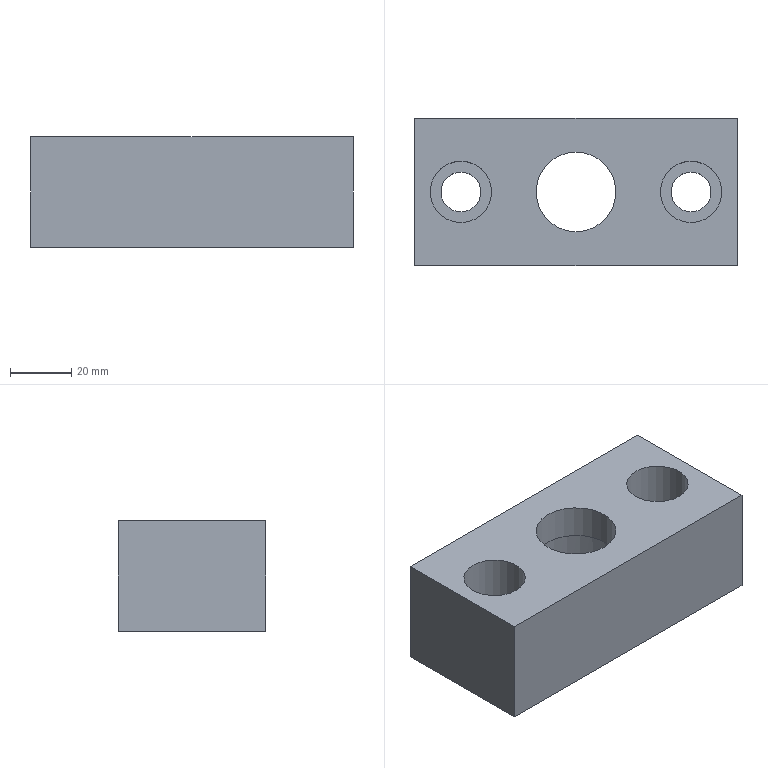Part | NX | features solid 2 | 1 solid | 15 faces | box 105 x 48 x 36 mm | volume 129547 mm3 | plane 9 | cylinder 6 | commonest cylinder face diameters 13 x2 20 x2 26 x1 40 x1
STEP:
#1=CARTESIAN_POINT('',(73.5,-257.,75.));
#2=VERTEX_POINT('',#1);
#3=CARTESIAN_POINT('',(73.5,-237.,75.));
#4=DIRECTION('',(0.,0.,1.));
#5=DIRECTION('',(0.,-1.,0.));
#6=AXIS2_PLACEMENT_3D('',#3,#4,#5);
#7=CIRCLE('',#6,20.);
#8=EDGE_CURVE('',#2,#2,#7,.F.);
#9=ORIENTED_EDGE('',*,*,#8,.T.);
#10=EDGE_LOOP('',(#9));
#11=FACE_BOUND('',#10,.T.);
#12=CARTESIAN_POINT('',(73.5,-250.,75.));
#13=VERTEX_POINT('',#12);
#14=CARTESIAN_POINT('',(73.5,-237.,75.));
#15=DIRECTION('',(0.,0.,1.));
#16=DIRECTION('',(0.,-1.,0.));
#17=AXIS2_PLACEMENT_3D('',#14,#15,#16);
#18=CIRCLE('',#17,13.);
#19=EDGE_CURVE('',#13,#13,#18,.F.);
#20=ORIENTED_EDGE('',*,*,#19,.F.);
#21=EDGE_LOOP('',(#20));
#22=FACE_BOUND('',#21,.T.);
#23=CARTESIAN_POINT('',(73.5,-219.,75.));
#24=DIRECTION('',(0.,0.,-1.));
#25=DIRECTION('',(0.,1.,0.));
#26=AXIS2_PLACEMENT_3D('',#23,#24,#25);
#27=PLANE('',#26);
#28=ADVANCED_FACE('',(#11,#22),#27,.T.);
#29=CARTESIAN_POINT('',(36.,-243.5,72.));
#30=VERTEX_POINT('',#29);
#31=CARTESIAN_POINT('',(36.,-237.,72.));
#32=DIRECTION('',(0.,0.,1.));
#33=DIRECTION('',(0.,-1.,0.));
#34=AXIS2_PLACEMENT_3D('',#31,#32,#33);
#35=CIRCLE('',#34,6.5);
#36=EDGE_CURVE('',#30,#30,#35,.F.);
#37=ORIENTED_EDGE('',*,*,#36,.T.);
#38=EDGE_LOOP('',(#37));
#39=FACE_BOUND('',#38,.T.);
#40=CARTESIAN_POINT('',(36.,-247.,72.));
#41=VERTEX_POINT('',#40);
#42=CARTESIAN_POINT('',(36.,-237.,72.));
#43=DIRECTION('',(0.,0.,1.));
#44=DIRECTION('',(0.,-1.,0.));
#45=AXIS2_PLACEMENT_3D('',#42,#43,#44);
#46=CIRCLE('',#45,10.);
#47=EDGE_CURVE('',#41,#41,#46,.F.);
#48=ORIENTED_EDGE('',*,*,#47,.F.);
#49=EDGE_LOOP('',(#48));
#50=FACE_BOUND('',#49,.T.);
#51=CARTESIAN_POINT('',(36.54,-237.447,72.));
#52=DIRECTION('',(0.,0.,-1.));
#53=DIRECTION('',(0.,-1.,0.));
#54=AXIS2_PLACEMENT_3D('',#51,#52,#53);
#55=PLANE('',#54);
#56=ADVANCED_FACE('',(#39,#50),#55,.F.);
#57=CARTESIAN_POINT('',(73.5,-224.,86.));
#58=VERTEX_POINT('',#57);
#59=CARTESIAN_POINT('',(73.5,-237.,86.));
#60=DIRECTION('',(0.,0.,-1.));
#61=DIRECTION('',(0.,1.,0.));
#62=AXIS2_PLACEMENT_3D('',#59,#60,#61);
#63=CIRCLE('',#62,13.);
#64=EDGE_CURVE('',#58,#58,#63,.F.);
#65=ORIENTED_EDGE('',*,*,#64,.T.);
#66=EDGE_LOOP('',(#65));
#67=FACE_BOUND('',#66,.T.);
#68=ORIENTED_EDGE('',*,*,#19,.T.);
#69=EDGE_LOOP('',(#68));
#70=FACE_BOUND('',#69,.T.);
#71=CARTESIAN_POINT('',(73.5,-237.,29.5));
#72=DIRECTION('',(0.,0.,1.));
#73=DIRECTION('',(0.,1.,0.));
#74=AXIS2_PLACEMENT_3D('',#71,#72,#73);
#75=CYLINDRICAL_SURFACE('',#74,13.);
#76=ADVANCED_FACE('',(#67,#70),#75,.F.);
#77=CARTESIAN_POINT('',(73.5,-217.,50.));
#78=VERTEX_POINT('',#77);
#79=CARTESIAN_POINT('',(73.5,-237.,50.));
#80=DIRECTION('',(0.,0.,-1.));
#81=DIRECTION('',(0.,1.,0.));
#82=AXIS2_PLACEMENT_3D('',#79,#80,#81);
#83=CIRCLE('',#82,20.);
#84=EDGE_CURVE('',#78,#78,#83,.T.);
#85=ORIENTED_EDGE('',*,*,#84,.T.);
#86=EDGE_LOOP('',(#85));
#87=FACE_BOUND('',#86,.T.);
#88=ORIENTED_EDGE('',*,*,#8,.F.);
#89=EDGE_LOOP('',(#88));
#90=FACE_BOUND('',#89,.T.);
#91=CARTESIAN_POINT('',(73.5,-237.,29.));
#92=DIRECTION('',(0.,0.,1.));
#93=DIRECTION('',(0.,1.,0.));
#94=AXIS2_PLACEMENT_3D('',#91,#92,#93);
#95=CYLINDRICAL_SURFACE('',#94,20.);
#96=ADVANCED_FACE('',(#87,#90),#95,.F.);
#97=CARTESIAN_POINT('',(126.,-261.,50.));
#98=VERTEX_POINT('',#97);
#99=CARTESIAN_POINT('',(126.,-261.,86.));
#100=VERTEX_POINT('',#99);
#101=CARTESIAN_POINT('',(126.,-261.,67.5));
#102=DIRECTION('',(0.,0.,1.));
#103=VECTOR('',#102,1000.);
#104=LINE('',#101,#103);
#105=EDGE_CURVE('',#98,#100,#104,.T.);
#106=ORIENTED_EDGE('',*,*,#105,.F.);
#107=CARTESIAN_POINT('',(126.,-213.,50.));
#108=VERTEX_POINT('',#107);
#109=CARTESIAN_POINT('',(126.,-237.,50.));
#110=DIRECTION('',(0.,1.,0.));
#111=VECTOR('',#110,1000.);
#112=LINE('',#109,#111);
#113=EDGE_CURVE('',#108,#98,#112,.F.);
#114=ORIENTED_EDGE('',*,*,#113,.F.);
#115=CARTESIAN_POINT('',(126.,-213.,86.));
#116=VERTEX_POINT('',#115);
#117=CARTESIAN_POINT('',(126.,-213.,67.5));
#118=DIRECTION('',(0.,0.,1.));
#119=VECTOR('',#118,1000.);
#120=LINE('',#117,#119);
#121=EDGE_CURVE('',#108,#116,#120,.T.);
#122=ORIENTED_EDGE('',*,*,#121,.T.);
#123=CARTESIAN_POINT('',(126.,-237.,86.));
#124=DIRECTION('',(0.,1.,0.));
#125=VECTOR('',#124,1000.);
#126=LINE('',#123,#125);
#127=EDGE_CURVE('',#100,#116,#126,.T.);
#128=ORIENTED_EDGE('',*,*,#127,.F.);
#129=EDGE_LOOP('',(#106,#114,#122,#128));
#130=FACE_BOUND('',#129,.T.);
#131=CARTESIAN_POINT('',(126.,-237.,67.5));
#132=DIRECTION('',(1.,0.,0.));
#133=DIRECTION('',(0.,0.,1.));
#134=AXIS2_PLACEMENT_3D('',#131,#132,#133);
#135=PLANE('',#134);
#136=ADVANCED_FACE('',(#130),#135,.T.);
#137=CARTESIAN_POINT('',(21.,-261.,50.));
#138=VERTEX_POINT('',#137);
#139=CARTESIAN_POINT('',(21.,-261.,86.));
#140=VERTEX_POINT('',#139);
#141=CARTESIAN_POINT('',(21.,-261.,67.5));
#142=DIRECTION('',(0.,0.,1.));
#143=VECTOR('',#142,1000.);
#144=LINE('',#141,#143);
#145=EDGE_CURVE('',#138,#140,#144,.T.);
#146=ORIENTED_EDGE('',*,*,#145,.F.);
#147=CARTESIAN_POINT('',(73.5,-261.,50.));
#148=DIRECTION('',(1.,0.,0.));
#149=VECTOR('',#148,1000.);
#150=LINE('',#147,#149);
#151=EDGE_CURVE('',#98,#138,#150,.F.);
#152=ORIENTED_EDGE('',*,*,#151,.F.);
#153=ORIENTED_EDGE('',*,*,#105,.T.);
#154=CARTESIAN_POINT('',(73.5,-261.,86.));
#155=DIRECTION('',(1.,0.,0.));
#156=VECTOR('',#155,1000.);
#157=LINE('',#154,#156);
#158=EDGE_CURVE('',#140,#100,#157,.T.);
#159=ORIENTED_EDGE('',*,*,#158,.F.);
#160=EDGE_LOOP('',(#146,#152,#153,#159));
#161=FACE_BOUND('',#160,.T.);
#162=CARTESIAN_POINT('',(73.5,-261.,67.5));
#163=DIRECTION('',(0.,-1.,0.));
#164=DIRECTION('',(0.,0.,1.));
#165=AXIS2_PLACEMENT_3D('',#162,#163,#164);
#166=PLANE('',#165);
#167=ADVANCED_FACE('',(#161),#166,.T.);
#168=CARTESIAN_POINT('',(21.,-213.,50.));
#169=VERTEX_POINT('',#168);
#170=CARTESIAN_POINT('',(21.,-213.,86.));
#171=VERTEX_POINT('',#170);
#172=CARTESIAN_POINT('',(21.,-213.,67.5));
#173=DIRECTION('',(0.,0.,1.));
#174=VECTOR('',#173,1000.);
#175=LINE('',#172,#174);
#176=EDGE_CURVE('',#169,#171,#175,.T.);
#177=ORIENTED_EDGE('',*,*,#176,.F.);
#178=CARTESIAN_POINT('',(21.,-237.,50.));
#179=DIRECTION('',(0.,-1.,0.));
#180=VECTOR('',#179,1000.);
#181=LINE('',#178,#180);
#182=EDGE_CURVE('',#138,#169,#181,.F.);
#183=ORIENTED_EDGE('',*,*,#182,.F.);
#184=ORIENTED_EDGE('',*,*,#145,.T.);
#185=CARTESIAN_POINT('',(21.,-237.,86.));
#186=DIRECTION('',(0.,-1.,0.));
#187=VECTOR('',#186,1000.);
#188=LINE('',#185,#187);
#189=EDGE_CURVE('',#171,#140,#188,.T.);
#190=ORIENTED_EDGE('',*,*,#189,.F.);
#191=EDGE_LOOP('',(#177,#183,#184,#190));
#192=FACE_BOUND('',#191,.T.);
#193=CARTESIAN_POINT('',(21.,-237.,67.5));
#194=DIRECTION('',(-1.,0.,0.));
#195=DIRECTION('',(0.,0.,-1.));
#196=AXIS2_PLACEMENT_3D('',#193,#194,#195);
#197=PLANE('',#196);
#198=ADVANCED_FACE('',(#192),#197,.T.);
#199=CARTESIAN_POINT('',(73.5,-213.,50.));
#200=DIRECTION('',(-1.,0.,0.));
#201=VECTOR('',#200,1000.);
#202=LINE('',#199,#201);
#203=EDGE_CURVE('',#169,#108,#202,.F.);
#204=ORIENTED_EDGE('',*,*,#203,.F.);
#205=ORIENTED_EDGE('',*,*,#176,.T.);
#206=CARTESIAN_POINT('',(73.5,-213.,86.));
#207=DIRECTION('',(-1.,0.,0.));
#208=VECTOR('',#207,1000.);
#209=LINE('',#206,#208);
#210=EDGE_CURVE('',#116,#171,#209,.T.);
#211=ORIENTED_EDGE('',*,*,#210,.F.);
#212=ORIENTED_EDGE('',*,*,#121,.F.);
#213=EDGE_LOOP('',(#204,#205,#211,#212));
#214=FACE_BOUND('',#213,.T.);
#215=CARTESIAN_POINT('',(73.5,-213.,67.5));
#216=DIRECTION('',(0.,1.,0.));
#217=DIRECTION('',(0.,0.,-1.));
#218=AXIS2_PLACEMENT_3D('',#215,#216,#217);
#219=PLANE('',#218);
#220=ADVANCED_FACE('',(#214),#219,.T.);
#221=CARTESIAN_POINT('',(36.,-230.5,50.));
#222=VERTEX_POINT('',#221);
#223=CARTESIAN_POINT('',(36.,-237.,50.));
#224=DIRECTION('',(0.,0.,-1.));
#225=DIRECTION('',(0.,1.,0.));
#226=AXIS2_PLACEMENT_3D('',#223,#224,#225);
#227=CIRCLE('',#226,6.5);
#228=EDGE_CURVE('',#222,#222,#227,.F.);
#229=ORIENTED_EDGE('',*,*,#228,.F.);
#230=EDGE_LOOP('',(#229));
#231=FACE_BOUND('',#230,.T.);
#232=ORIENTED_EDGE('',*,*,#36,.F.);
#233=EDGE_LOOP('',(#232));
#234=FACE_BOUND('',#233,.T.);
#235=CARTESIAN_POINT('',(36.,-237.,36.));
#236=DIRECTION('',(0.,0.,-1.));
#237=DIRECTION('',(0.,-1.,0.));
#238=AXIS2_PLACEMENT_3D('',#235,#236,#237);
#239=CYLINDRICAL_SURFACE('',#238,6.5);
#240=ADVANCED_FACE('',(#231,#234),#239,.F.);
#241=CARTESIAN_POINT('',(111.,-230.5,50.));
#242=VERTEX_POINT('',#241);
#243=CARTESIAN_POINT('',(111.,-237.,50.));
#244=DIRECTION('',(0.,0.,-1.));
#245=DIRECTION('',(0.,1.,0.));
#246=AXIS2_PLACEMENT_3D('',#243,#244,#245);
#247=CIRCLE('',#246,6.5);
#248=EDGE_CURVE('',#242,#242,#247,.F.);
#249=ORIENTED_EDGE('',*,*,#248,.T.);
#250=EDGE_LOOP('',(#249));
#251=FACE_BOUND('',#250,.T.);
#252=ORIENTED_EDGE('',*,*,#228,.T.);
#253=EDGE_LOOP('',(#252));
#254=FACE_BOUND('',#253,.T.);
#255=ORIENTED_EDGE('',*,*,#203,.T.);
#256=ORIENTED_EDGE('',*,*,#113,.T.);
#257=ORIENTED_EDGE('',*,*,#151,.T.);
#258=ORIENTED_EDGE('',*,*,#182,.T.);
#259=EDGE_LOOP('',(#255,#256,#257,#258));
#260=FACE_BOUND('',#259,.T.);
#261=ORIENTED_EDGE('',*,*,#84,.F.);
#262=EDGE_LOOP('',(#261));
#263=FACE_BOUND('',#262,.T.);
#264=CARTESIAN_POINT('',(-296.5,11.379,50.));
#265=DIRECTION('',(0.,0.,1.));
#266=DIRECTION('',(0.,1.,0.));
#267=AXIS2_PLACEMENT_3D('',#264,#265,#266);
#268=PLANE('',#267);
#269=ADVANCED_FACE('',(#251,#254,#260,#263),#268,.F.);
#270=ORIENTED_EDGE('',*,*,#47,.T.);
#271=EDGE_LOOP('',(#270));
#272=FACE_BOUND('',#271,.T.);
#273=CARTESIAN_POINT('',(36.,-247.,86.));
#274=VERTEX_POINT('',#273);
#275=CARTESIAN_POINT('',(36.,-237.,86.));
#276=DIRECTION('',(0.,0.,1.));
#277=DIRECTION('',(0.,-1.,0.));
#278=AXIS2_PLACEMENT_3D('',#275,#276,#277);
#279=CIRCLE('',#278,10.);
#280=EDGE_CURVE('',#274,#274,#279,.T.);
#281=ORIENTED_EDGE('',*,*,#280,.T.);
#282=EDGE_LOOP('',(#281));
#283=FACE_BOUND('',#282,.T.);
#284=CARTESIAN_POINT('',(36.,-237.,86.));
#285=DIRECTION('',(0.,0.,-1.));
#286=DIRECTION('',(0.,-1.,0.));
#287=AXIS2_PLACEMENT_3D('',#284,#285,#286);
#288=CYLINDRICAL_SURFACE('',#287,10.);
#289=ADVANCED_FACE('',(#272,#283),#288,.F.);
#290=CARTESIAN_POINT('',(111.,-227.,86.));
#291=VERTEX_POINT('',#290);
#292=CARTESIAN_POINT('',(111.,-237.,86.));
#293=DIRECTION('',(0.,0.,-1.));
#294=DIRECTION('',(0.,1.,0.));
#295=AXIS2_PLACEMENT_3D('',#292,#293,#294);
#296=CIRCLE('',#295,10.);
#297=EDGE_CURVE('',#291,#291,#296,.T.);
#298=ORIENTED_EDGE('',*,*,#297,.T.);
#299=EDGE_LOOP('',(#298));
#300=FACE_BOUND('',#299,.T.);
#301=ORIENTED_EDGE('',*,*,#280,.F.);
#302=EDGE_LOOP('',(#301));
#303=FACE_BOUND('',#302,.T.);
#304=ORIENTED_EDGE('',*,*,#189,.T.);
#305=ORIENTED_EDGE('',*,*,#158,.T.);
#306=ORIENTED_EDGE('',*,*,#127,.T.);
#307=ORIENTED_EDGE('',*,*,#210,.T.);
#308=EDGE_LOOP('',(#304,#305,#306,#307));
#309=FACE_BOUND('',#308,.T.);
#310=ORIENTED_EDGE('',*,*,#64,.F.);
#311=EDGE_LOOP('',(#310));
#312=FACE_BOUND('',#311,.T.);
#313=CARTESIAN_POINT('',(-211.5,11.379,86.));
#314=DIRECTION('',(0.,0.,1.));
#315=DIRECTION('',(0.,-1.,0.));
#316=AXIS2_PLACEMENT_3D('',#313,#314,#315);
#317=PLANE('',#316);
#318=ADVANCED_FACE('',(#300,#303,#309,#312),#317,.T.);
#319=CARTESIAN_POINT('',(111.,-243.5,72.));
#320=VERTEX_POINT('',#319);
#321=CARTESIAN_POINT('',(111.,-237.,72.));
#322=DIRECTION('',(0.,0.,-1.));
#323=DIRECTION('',(0.,-1.,0.));
#324=AXIS2_PLACEMENT_3D('',#321,#322,#323);
#325=CIRCLE('',#324,6.5);
#326=EDGE_CURVE('',#320,#320,#325,.T.);
#327=ORIENTED_EDGE('',*,*,#326,.T.);
#328=EDGE_LOOP('',(#327));
#329=FACE_BOUND('',#328,.T.);
#330=CARTESIAN_POINT('',(111.,-247.,72.));
#331=VERTEX_POINT('',#330);
#332=CARTESIAN_POINT('',(111.,-237.,72.));
#333=DIRECTION('',(0.,0.,-1.));
#334=DIRECTION('',(0.,-1.,0.));
#335=AXIS2_PLACEMENT_3D('',#332,#333,#334);
#336=CIRCLE('',#335,10.);
#337=EDGE_CURVE('',#331,#331,#336,.T.);
#338=ORIENTED_EDGE('',*,*,#337,.F.);
#339=EDGE_LOOP('',(#338));
#340=FACE_BOUND('',#339,.T.);
#341=CARTESIAN_POINT('',(110.46,-237.447,72.));
#342=DIRECTION('',(0.,0.,-1.));
#343=DIRECTION('',(0.,-1.,0.));
#344=AXIS2_PLACEMENT_3D('',#341,#342,#343);
#345=PLANE('',#344);
#346=ADVANCED_FACE('',(#329,#340),#345,.F.);
#347=ORIENTED_EDGE('',*,*,#248,.F.);
#348=EDGE_LOOP('',(#347));
#349=FACE_BOUND('',#348,.T.);
#350=ORIENTED_EDGE('',*,*,#326,.F.);
#351=EDGE_LOOP('',(#350));
#352=FACE_BOUND('',#351,.T.);
#353=CARTESIAN_POINT('',(111.,-237.,36.));
#354=DIRECTION('',(0.,0.,-1.));
#355=DIRECTION('',(0.,-1.,0.));
#356=AXIS2_PLACEMENT_3D('',#353,#354,#355);
#357=CYLINDRICAL_SURFACE('',#356,6.5);
#358=ADVANCED_FACE('',(#349,#352),#357,.F.);
#359=ORIENTED_EDGE('',*,*,#337,.T.);
#360=EDGE_LOOP('',(#359));
#361=FACE_BOUND('',#360,.T.);
#362=ORIENTED_EDGE('',*,*,#297,.F.);
#363=EDGE_LOOP('',(#362));
#364=FACE_BOUND('',#363,.T.);
#365=CARTESIAN_POINT('',(111.,-237.,86.));
#366=DIRECTION('',(0.,0.,-1.));
#367=DIRECTION('',(0.,-1.,0.));
#368=AXIS2_PLACEMENT_3D('',#365,#366,#367);
#369=CYLINDRICAL_SURFACE('',#368,10.);
#370=ADVANCED_FACE('',(#361,#364),#369,.F.);
#371=CLOSED_SHELL('',(#28,#56,#76,#96,#136,#167,#198,#220,#240,#269,#289,#318,#346,#358,#370));
#372=MANIFOLD_SOLID_BREP('',#371);
#373=(LENGTH_UNIT()NAMED_UNIT(*)SI_UNIT(.MILLI.,.METRE.));
#374=UNCERTAINTY_MEASURE_WITH_UNIT(LENGTH_MEASURE(0.00001),#373,'','');
#375=(NAMED_UNIT(*)PLANE_ANGLE_UNIT()SI_UNIT($,.RADIAN.));
#376=(NAMED_UNIT(*)SI_UNIT($,.STERADIAN.)SOLID_ANGLE_UNIT());
#377=(GEOMETRIC_REPRESENTATION_CONTEXT(3)GLOBAL_UNCERTAINTY_ASSIGNED_CONTEXT((#374))GLOBAL_UNIT_ASSIGNED_CONTEXT((#373,#375,#376))REPRESENTATION_CONTEXT('',''));
#378=ADVANCED_BREP_SHAPE_REPRESENTATION('',(#372),#377);